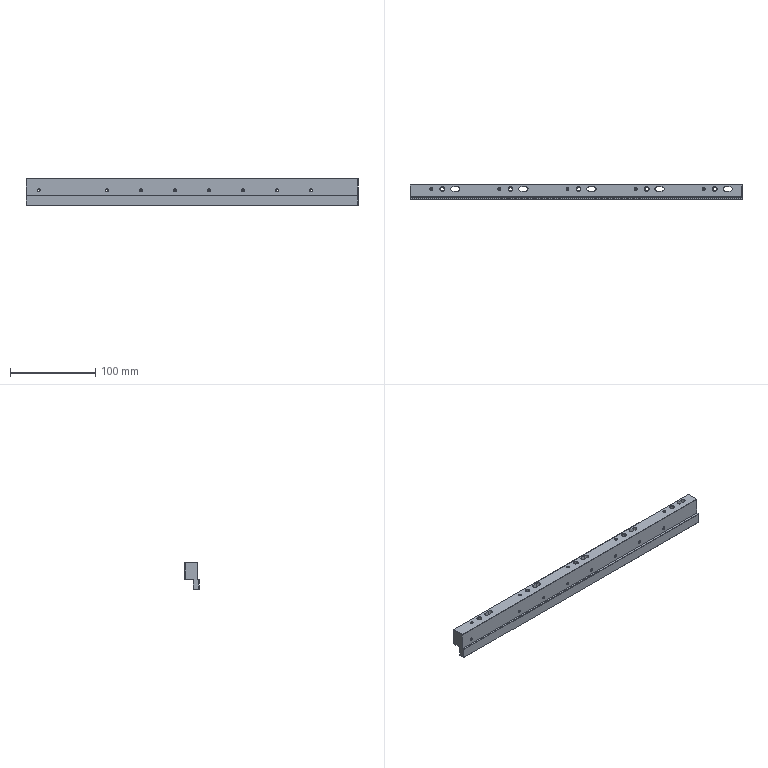Part | NX | 1 solid | 129 faces | box 390 x 17 x 32 mm | volume 138280 mm3 | cylinder 57 | plane 36 | cone 36 | commonest cylinder face diameters 2.5 x32 5.2 x15 4.2 x10